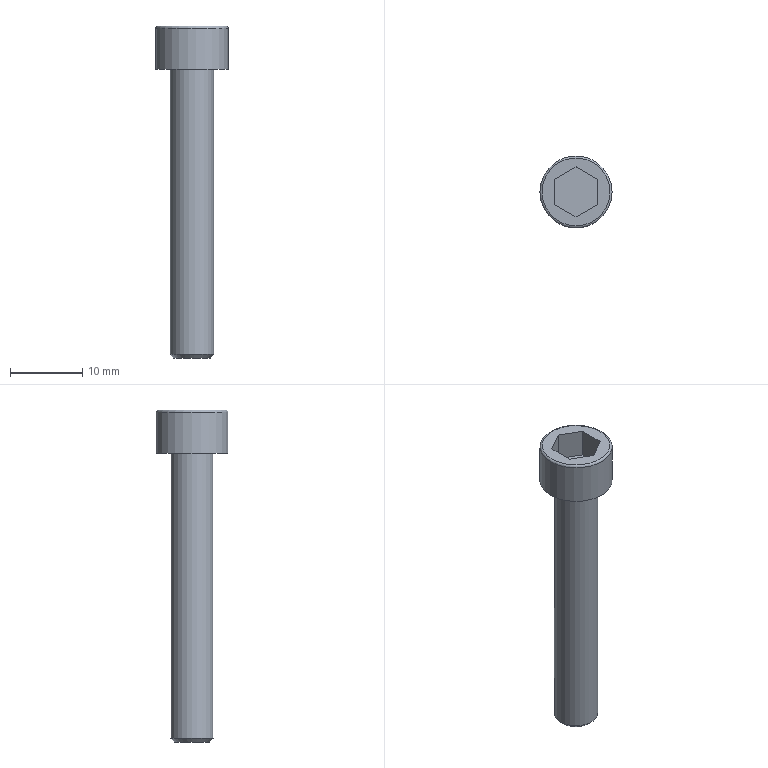Part | STEP file | 200 mesh_id670_x | 1 solid | 14 faces | box 10 x 10 x 46 mm | volume 1475 mm3 | plane 10 | cylinder 2 | torus 1 | cone 1 | commonest cylinder face diameters 6 x1 10 x1
STEP:
#1=CARTESIAN_POINT('',(-16712.686,-4170.269,-13.5));
#2=VERTEX_POINT('',#1);
#3=CARTESIAN_POINT('',(-16709.686,-4170.269,-13.5));
#4=DIRECTION('',(0.,0.,1.));
#5=DIRECTION('',(-1.,0.,0.));
#6=AXIS2_PLACEMENT_3D('',#3,#4,#5);
#7=CIRCLE('',#6,3.);
#8=EDGE_CURVE('',#2,#2,#7,.T.);
#9=ORIENTED_EDGE('',*,*,#8,.T.);
#10=EDGE_LOOP('',(#9));
#11=FACE_BOUND('',#10,.T.);
#12=CARTESIAN_POINT('',(-16712.686,-4170.269,26.));
#13=VERTEX_POINT('',#12);
#14=CARTESIAN_POINT('',(-16709.686,-4170.269,26.));
#15=DIRECTION('',(0.,0.,1.));
#16=DIRECTION('',(-1.,0.,0.));
#17=AXIS2_PLACEMENT_3D('',#14,#15,#16);
#18=CIRCLE('',#17,3.);
#19=EDGE_CURVE('',#13,#13,#18,.T.);
#20=ORIENTED_EDGE('',*,*,#19,.F.);
#21=EDGE_LOOP('',(#20));
#22=FACE_BOUND('',#21,.T.);
#23=CARTESIAN_POINT('',(-16709.686,-4170.269,26.));
#24=DIRECTION('',(0.,0.,-1.));
#25=DIRECTION('',(1.,0.,0.));
#26=AXIS2_PLACEMENT_3D('',#23,#24,#25);
#27=CYLINDRICAL_SURFACE('',#26,3.);
#28=ADVANCED_FACE('',(#11,#22),#27,.T.);
#29=CARTESIAN_POINT('',(-16704.986,-4170.269,32.));
#30=VERTEX_POINT('',#29);
#31=CARTESIAN_POINT('',(-16709.686,-4170.269,32.));
#32=DIRECTION('',(0.,0.,1.));
#33=DIRECTION('',(1.,0.,0.));
#34=AXIS2_PLACEMENT_3D('',#31,#32,#33);
#35=CIRCLE('',#34,4.7);
#36=EDGE_CURVE('',#30,#30,#35,.T.);
#37=ORIENTED_EDGE('',*,*,#36,.T.);
#38=EDGE_LOOP('',(#37));
#39=FACE_BOUND('',#38,.T.);
#40=CARTESIAN_POINT('',(-16712.686,-4168.537,32.));
#41=VERTEX_POINT('',#40);
#42=CARTESIAN_POINT('',(-16712.686,-4172.001,32.));
#43=VERTEX_POINT('',#42);
#44=CARTESIAN_POINT('',(-16712.686,-4168.537,32.));
#45=DIRECTION('',(0.,-1.,0.));
#46=VECTOR('',#45,1.);
#47=LINE('',#44,#46);
#48=EDGE_CURVE('',#41,#43,#47,.T.);
#49=ORIENTED_EDGE('',*,*,#48,.F.);
#50=CARTESIAN_POINT('',(-16709.686,-4166.805,32.));
#51=VERTEX_POINT('',#50);
#52=CARTESIAN_POINT('',(-16709.686,-4166.805,32.));
#53=DIRECTION('',(-0.866,-0.5,0.));
#54=VECTOR('',#53,1.);
#55=LINE('',#52,#54);
#56=EDGE_CURVE('',#51,#41,#55,.T.);
#57=ORIENTED_EDGE('',*,*,#56,.F.);
#58=CARTESIAN_POINT('',(-16706.686,-4168.537,32.));
#59=VERTEX_POINT('',#58);
#60=CARTESIAN_POINT('',(-16706.686,-4168.537,32.));
#61=DIRECTION('',(-0.866,0.5,0.));
#62=VECTOR('',#61,1.);
#63=LINE('',#60,#62);
#64=EDGE_CURVE('',#59,#51,#63,.T.);
#65=ORIENTED_EDGE('',*,*,#64,.F.);
#66=CARTESIAN_POINT('',(-16706.686,-4172.001,32.));
#67=VERTEX_POINT('',#66);
#68=CARTESIAN_POINT('',(-16706.686,-4172.001,32.));
#69=DIRECTION('',(0.,1.,0.));
#70=VECTOR('',#69,1.);
#71=LINE('',#68,#70);
#72=EDGE_CURVE('',#67,#59,#71,.T.);
#73=ORIENTED_EDGE('',*,*,#72,.F.);
#74=CARTESIAN_POINT('',(-16709.686,-4173.733,32.));
#75=VERTEX_POINT('',#74);
#76=CARTESIAN_POINT('',(-16709.686,-4173.733,32.));
#77=DIRECTION('',(0.866,0.5,0.));
#78=VECTOR('',#77,1.);
#79=LINE('',#76,#78);
#80=EDGE_CURVE('',#75,#67,#79,.T.);
#81=ORIENTED_EDGE('',*,*,#80,.F.);
#82=CARTESIAN_POINT('',(-16712.686,-4172.001,32.));
#83=DIRECTION('',(0.866,-0.5,0.));
#84=VECTOR('',#83,1.);
#85=LINE('',#82,#84);
#86=EDGE_CURVE('',#43,#75,#85,.T.);
#87=ORIENTED_EDGE('',*,*,#86,.F.);
#88=EDGE_LOOP('',(#49,#57,#65,#73,#81,#87));
#89=FACE_BOUND('',#88,.T.);
#90=CARTESIAN_POINT('',(-16709.686,-4170.269,32.));
#91=DIRECTION('',(0.,0.,1.));
#92=DIRECTION('',(1.,0.,0.));
#93=AXIS2_PLACEMENT_3D('',#90,#91,#92);
#94=PLANE('',#93);
#95=ADVANCED_FACE('',(#39,#89),#94,.T.);
#96=ORIENTED_EDGE('',*,*,#19,.T.);
#97=EDGE_LOOP('',(#96));
#98=FACE_BOUND('',#97,.T.);
#99=CARTESIAN_POINT('',(-16704.686,-4170.269,26.));
#100=VERTEX_POINT('',#99);
#101=CARTESIAN_POINT('',(-16709.686,-4170.269,26.));
#102=DIRECTION('',(0.,0.,1.));
#103=DIRECTION('',(1.,0.,0.));
#104=AXIS2_PLACEMENT_3D('',#101,#102,#103);
#105=CIRCLE('',#104,5.);
#106=EDGE_CURVE('',#100,#100,#105,.T.);
#107=ORIENTED_EDGE('',*,*,#106,.F.);
#108=EDGE_LOOP('',(#107));
#109=FACE_BOUND('',#108,.T.);
#110=CARTESIAN_POINT('',(-16709.686,-4170.269,26.));
#111=DIRECTION('',(0.,0.,-1.));
#112=DIRECTION('',(-1.,0.,0.));
#113=AXIS2_PLACEMENT_3D('',#110,#111,#112);
#114=PLANE('',#113);
#115=ADVANCED_FACE('',(#98,#109),#114,.T.);
#116=CARTESIAN_POINT('',(-16704.686,-4170.269,31.7));
#117=VERTEX_POINT('',#116);
#118=CARTESIAN_POINT('',(-16709.686,-4170.269,31.7));
#119=DIRECTION('',(0.,0.,-1.));
#120=DIRECTION('',(1.,0.,0.));
#121=AXIS2_PLACEMENT_3D('',#118,#119,#120);
#122=CIRCLE('',#121,5.);
#123=EDGE_CURVE('',#117,#117,#122,.T.);
#124=ORIENTED_EDGE('',*,*,#123,.T.);
#125=EDGE_LOOP('',(#124));
#126=FACE_BOUND('',#125,.T.);
#127=ORIENTED_EDGE('',*,*,#106,.T.);
#128=EDGE_LOOP('',(#127));
#129=FACE_BOUND('',#128,.T.);
#130=CARTESIAN_POINT('',(-16709.686,-4170.269,26.));
#131=DIRECTION('',(0.,0.,1.));
#132=DIRECTION('',(1.,0.,0.));
#133=AXIS2_PLACEMENT_3D('',#130,#131,#132);
#134=CYLINDRICAL_SURFACE('',#133,5.);
#135=ADVANCED_FACE('',(#126,#129),#134,.T.);
#136=CARTESIAN_POINT('',(-16712.686,-4172.001,28.));
#137=VERTEX_POINT('',#136);
#138=CARTESIAN_POINT('',(-16712.686,-4168.537,28.));
#139=VERTEX_POINT('',#138);
#140=CARTESIAN_POINT('',(-16712.686,-4168.537,28.));
#141=DIRECTION('',(0.,1.,0.));
#142=VECTOR('',#141,1.);
#143=LINE('',#140,#142);
#144=EDGE_CURVE('',#137,#139,#143,.T.);
#145=ORIENTED_EDGE('',*,*,#144,.T.);
#146=CARTESIAN_POINT('',(-16712.686,-4168.537,32.));
#147=DIRECTION('',(0.,0.,1.));
#148=VECTOR('',#147,1.);
#149=LINE('',#146,#148);
#150=EDGE_CURVE('',#139,#41,#149,.T.);
#151=ORIENTED_EDGE('',*,*,#150,.T.);
#152=ORIENTED_EDGE('',*,*,#48,.T.);
#153=CARTESIAN_POINT('',(-16712.686,-4172.001,32.));
#154=DIRECTION('',(0.,0.,1.));
#155=VECTOR('',#154,1.);
#156=LINE('',#153,#155);
#157=EDGE_CURVE('',#137,#43,#156,.T.);
#158=ORIENTED_EDGE('',*,*,#157,.F.);
#159=EDGE_LOOP('',(#145,#151,#152,#158));
#160=FACE_OUTER_BOUND('',#159,.T.);
#161=CARTESIAN_POINT('',(-16712.686,-4168.537,32.));
#162=DIRECTION('',(1.,0.,0.));
#163=DIRECTION('',(0.,0.,-1.));
#164=AXIS2_PLACEMENT_3D('',#161,#162,#163);
#165=PLANE('',#164);
#166=ADVANCED_FACE('',(#160),#165,.T.);
#167=CARTESIAN_POINT('',(-16709.686,-4173.733,28.));
#168=VERTEX_POINT('',#167);
#169=CARTESIAN_POINT('',(-16712.686,-4172.001,28.));
#170=DIRECTION('',(-0.866,0.5,0.));
#171=VECTOR('',#170,1.);
#172=LINE('',#169,#171);
#173=EDGE_CURVE('',#168,#137,#172,.T.);
#174=ORIENTED_EDGE('',*,*,#173,.T.);
#175=ORIENTED_EDGE('',*,*,#157,.T.);
#176=ORIENTED_EDGE('',*,*,#86,.T.);
#177=CARTESIAN_POINT('',(-16709.686,-4173.733,32.));
#178=DIRECTION('',(0.,0.,1.));
#179=VECTOR('',#178,1.);
#180=LINE('',#177,#179);
#181=EDGE_CURVE('',#168,#75,#180,.T.);
#182=ORIENTED_EDGE('',*,*,#181,.F.);
#183=EDGE_LOOP('',(#174,#175,#176,#182));
#184=FACE_OUTER_BOUND('',#183,.T.);
#185=CARTESIAN_POINT('',(-16712.686,-4172.001,32.));
#186=DIRECTION('',(0.5,0.866,0.));
#187=DIRECTION('',(-0.866,0.5,0.));
#188=AXIS2_PLACEMENT_3D('',#185,#186,#187);
#189=PLANE('',#188);
#190=ADVANCED_FACE('',(#184),#189,.T.);
#191=CARTESIAN_POINT('',(-16706.686,-4172.001,28.));
#192=VERTEX_POINT('',#191);
#193=CARTESIAN_POINT('',(-16709.686,-4173.733,28.));
#194=DIRECTION('',(-0.866,-0.5,0.));
#195=VECTOR('',#194,1.);
#196=LINE('',#193,#195);
#197=EDGE_CURVE('',#192,#168,#196,.T.);
#198=ORIENTED_EDGE('',*,*,#197,.T.);
#199=ORIENTED_EDGE('',*,*,#181,.T.);
#200=ORIENTED_EDGE('',*,*,#80,.T.);
#201=CARTESIAN_POINT('',(-16706.686,-4172.001,32.));
#202=DIRECTION('',(0.,0.,1.));
#203=VECTOR('',#202,1.);
#204=LINE('',#201,#203);
#205=EDGE_CURVE('',#192,#67,#204,.T.);
#206=ORIENTED_EDGE('',*,*,#205,.F.);
#207=EDGE_LOOP('',(#198,#199,#200,#206));
#208=FACE_OUTER_BOUND('',#207,.T.);
#209=CARTESIAN_POINT('',(-16709.686,-4173.733,32.));
#210=DIRECTION('',(-0.5,0.866,0.));
#211=DIRECTION('',(-0.866,-0.5,0.));
#212=AXIS2_PLACEMENT_3D('',#209,#210,#211);
#213=PLANE('',#212);
#214=ADVANCED_FACE('',(#208),#213,.T.);
#215=CARTESIAN_POINT('',(-16706.686,-4168.537,28.));
#216=VERTEX_POINT('',#215);
#217=CARTESIAN_POINT('',(-16706.686,-4172.001,28.));
#218=DIRECTION('',(0.,-1.,0.));
#219=VECTOR('',#218,1.);
#220=LINE('',#217,#219);
#221=EDGE_CURVE('',#216,#192,#220,.T.);
#222=ORIENTED_EDGE('',*,*,#221,.T.);
#223=ORIENTED_EDGE('',*,*,#205,.T.);
#224=ORIENTED_EDGE('',*,*,#72,.T.);
#225=CARTESIAN_POINT('',(-16706.686,-4168.537,32.));
#226=DIRECTION('',(0.,0.,1.));
#227=VECTOR('',#226,1.);
#228=LINE('',#225,#227);
#229=EDGE_CURVE('',#216,#59,#228,.T.);
#230=ORIENTED_EDGE('',*,*,#229,.F.);
#231=EDGE_LOOP('',(#222,#223,#224,#230));
#232=FACE_OUTER_BOUND('',#231,.T.);
#233=CARTESIAN_POINT('',(-16706.686,-4172.001,32.));
#234=DIRECTION('',(-1.,0.,0.));
#235=DIRECTION('',(0.,0.,1.));
#236=AXIS2_PLACEMENT_3D('',#233,#234,#235);
#237=PLANE('',#236);
#238=ADVANCED_FACE('',(#232),#237,.T.);
#239=CARTESIAN_POINT('',(-16709.686,-4166.805,28.));
#240=VERTEX_POINT('',#239);
#241=CARTESIAN_POINT('',(-16706.686,-4168.537,28.));
#242=DIRECTION('',(0.866,-0.5,0.));
#243=VECTOR('',#242,1.);
#244=LINE('',#241,#243);
#245=EDGE_CURVE('',#240,#216,#244,.T.);
#246=ORIENTED_EDGE('',*,*,#245,.T.);
#247=ORIENTED_EDGE('',*,*,#229,.T.);
#248=ORIENTED_EDGE('',*,*,#64,.T.);
#249=CARTESIAN_POINT('',(-16709.686,-4166.805,32.));
#250=DIRECTION('',(0.,0.,1.));
#251=VECTOR('',#250,1.);
#252=LINE('',#249,#251);
#253=EDGE_CURVE('',#240,#51,#252,.T.);
#254=ORIENTED_EDGE('',*,*,#253,.F.);
#255=EDGE_LOOP('',(#246,#247,#248,#254));
#256=FACE_OUTER_BOUND('',#255,.T.);
#257=CARTESIAN_POINT('',(-16706.686,-4168.537,32.));
#258=DIRECTION('',(-0.5,-0.866,0.));
#259=DIRECTION('',(0.866,-0.5,0.));
#260=AXIS2_PLACEMENT_3D('',#257,#258,#259);
#261=PLANE('',#260);
#262=ADVANCED_FACE('',(#256),#261,.T.);
#263=CARTESIAN_POINT('',(-16709.686,-4166.805,28.));
#264=DIRECTION('',(0.866,0.5,0.));
#265=VECTOR('',#264,1.);
#266=LINE('',#263,#265);
#267=EDGE_CURVE('',#139,#240,#266,.T.);
#268=ORIENTED_EDGE('',*,*,#267,.T.);
#269=ORIENTED_EDGE('',*,*,#253,.T.);
#270=ORIENTED_EDGE('',*,*,#56,.T.);
#271=ORIENTED_EDGE('',*,*,#150,.F.);
#272=EDGE_LOOP('',(#268,#269,#270,#271));
#273=FACE_OUTER_BOUND('',#272,.T.);
#274=CARTESIAN_POINT('',(-16709.686,-4166.805,32.));
#275=DIRECTION('',(0.5,-0.866,0.));
#276=DIRECTION('',(0.866,0.5,0.));
#277=AXIS2_PLACEMENT_3D('',#274,#275,#276);
#278=PLANE('',#277);
#279=ADVANCED_FACE('',(#273),#278,.T.);
#280=ORIENTED_EDGE('',*,*,#144,.F.);
#281=ORIENTED_EDGE('',*,*,#173,.F.);
#282=ORIENTED_EDGE('',*,*,#197,.F.);
#283=ORIENTED_EDGE('',*,*,#221,.F.);
#284=ORIENTED_EDGE('',*,*,#245,.F.);
#285=ORIENTED_EDGE('',*,*,#267,.F.);
#286=EDGE_LOOP('',(#280,#281,#282,#283,#284,#285));
#287=FACE_OUTER_BOUND('',#286,.T.);
#288=CARTESIAN_POINT('',(0.,0.,28.));
#289=DIRECTION('',(0.,0.,1.));
#290=DIRECTION('',(1.,0.,0.));
#291=AXIS2_PLACEMENT_3D('',#288,#289,#290);
#292=PLANE('',#291);
#293=ADVANCED_FACE('',(#287),#292,.T.);
#294=ORIENTED_EDGE('',*,*,#36,.F.);
#295=EDGE_LOOP('',(#294));
#296=FACE_BOUND('',#295,.T.);
#297=ORIENTED_EDGE('',*,*,#123,.F.);
#298=EDGE_LOOP('',(#297));
#299=FACE_BOUND('',#298,.T.);
#300=CARTESIAN_POINT('',(-16709.686,-4170.269,31.7));
#301=DIRECTION('',(0.,0.,1.));
#302=DIRECTION('',(1.,0.,0.));
#303=AXIS2_PLACEMENT_3D('',#300,#301,#302);
#304=TOROIDAL_SURFACE('',#303,4.7,0.3);
#305=ADVANCED_FACE('',(#296,#299),#304,.T.);
#306=CARTESIAN_POINT('',(-16712.186,-4170.269,-14.));
#307=VERTEX_POINT('',#306);
#308=CARTESIAN_POINT('',(-16709.686,-4170.269,-14.));
#309=DIRECTION('',(0.,0.,-1.));
#310=DIRECTION('',(-1.,0.,0.));
#311=AXIS2_PLACEMENT_3D('',#308,#309,#310);
#312=CIRCLE('',#311,2.5);
#313=EDGE_CURVE('',#307,#307,#312,.T.);
#314=ORIENTED_EDGE('',*,*,#313,.T.);
#315=EDGE_LOOP('',(#314));
#316=FACE_OUTER_BOUND('',#315,.T.);
#317=CARTESIAN_POINT('',(-16709.686,-4170.269,-14.));
#318=DIRECTION('',(0.,0.,-1.));
#319=DIRECTION('',(-1.,0.,0.));
#320=AXIS2_PLACEMENT_3D('',#317,#318,#319);
#321=PLANE('',#320);
#322=ADVANCED_FACE('',(#316),#321,.T.);
#323=ORIENTED_EDGE('',*,*,#313,.F.);
#324=EDGE_LOOP('',(#323));
#325=FACE_BOUND('',#324,.T.);
#326=ORIENTED_EDGE('',*,*,#8,.F.);
#327=EDGE_LOOP('',(#326));
#328=FACE_BOUND('',#327,.T.);
#329=CARTESIAN_POINT('',(-16709.686,-4170.269,-13.5));
#330=DIRECTION('',(0.,0.,1.));
#331=DIRECTION('',(1.,0.,0.));
#332=AXIS2_PLACEMENT_3D('',#329,#330,#331);
#333=CONICAL_SURFACE('',#332,3.,45.);
#334=ADVANCED_FACE('',(#325,#328),#333,.T.);
#335=CLOSED_SHELL('',(#28,#95,#115,#135,#166,#190,#214,#238,#262,#279,#293,#305,#322,#334));
#336=MANIFOLD_SOLID_BREP('',#335);
#337=(LENGTH_UNIT()NAMED_UNIT(*)SI_UNIT(.MILLI.,.METRE.));
#338=UNCERTAINTY_MEASURE_WITH_UNIT(LENGTH_MEASURE(0.00002),#337,'','');
#339=(NAMED_UNIT(*)PLANE_ANGLE_UNIT()SI_UNIT($,.RADIAN.));
#340=PLANE_ANGLE_MEASURE_WITH_UNIT(PLANE_ANGLE_MEASURE(0.01745),#339);
#341=DIMENSIONAL_EXPONENTS(0.,0.,0.,0.,0.,0.,0.);
#342=(CONVERSION_BASED_UNIT('DEGREE',#340)NAMED_UNIT(#341)PLANE_ANGLE_UNIT());
#343=(NAMED_UNIT(*)SI_UNIT($,.STERADIAN.)SOLID_ANGLE_UNIT());
#344=(GEOMETRIC_REPRESENTATION_CONTEXT(3)GLOBAL_UNCERTAINTY_ASSIGNED_CONTEXT((#338))GLOBAL_UNIT_ASSIGNED_CONTEXT((#337,#342,#343))REPRESENTATION_CONTEXT('',''));
#345=ADVANCED_BREP_SHAPE_REPRESENTATION('',(#336),#344);